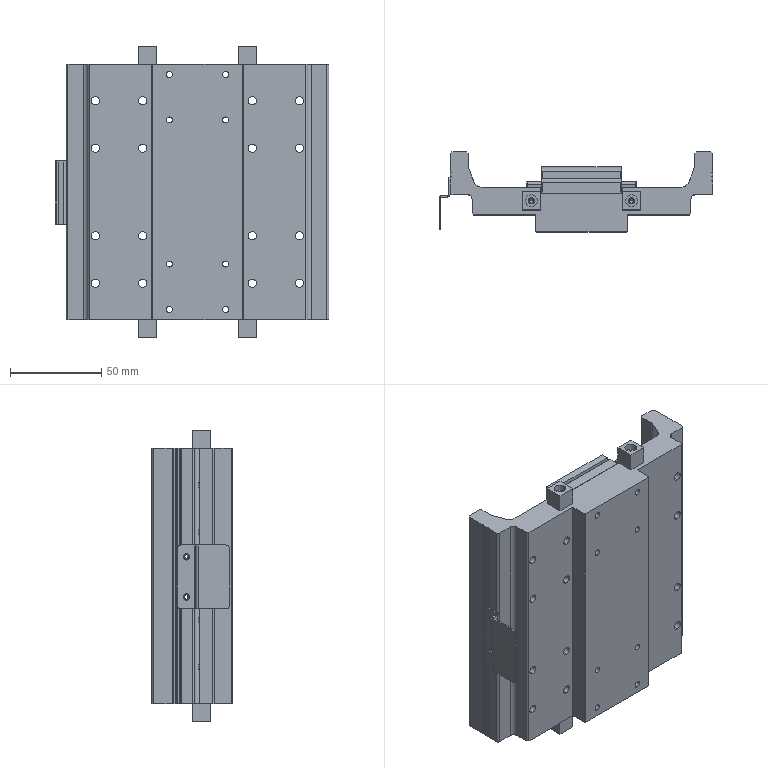Part | SolidWorks | 12 solids | 557 faces | box 150 x 44 x 160 mm | volume 393138 mm3 | cylinder 296 | plane 212 | cone 49 | commonest cylinder face diameters 8 x50 1 x48 4.5 x48 6.522 x22 2.5 x20 3.3 x16